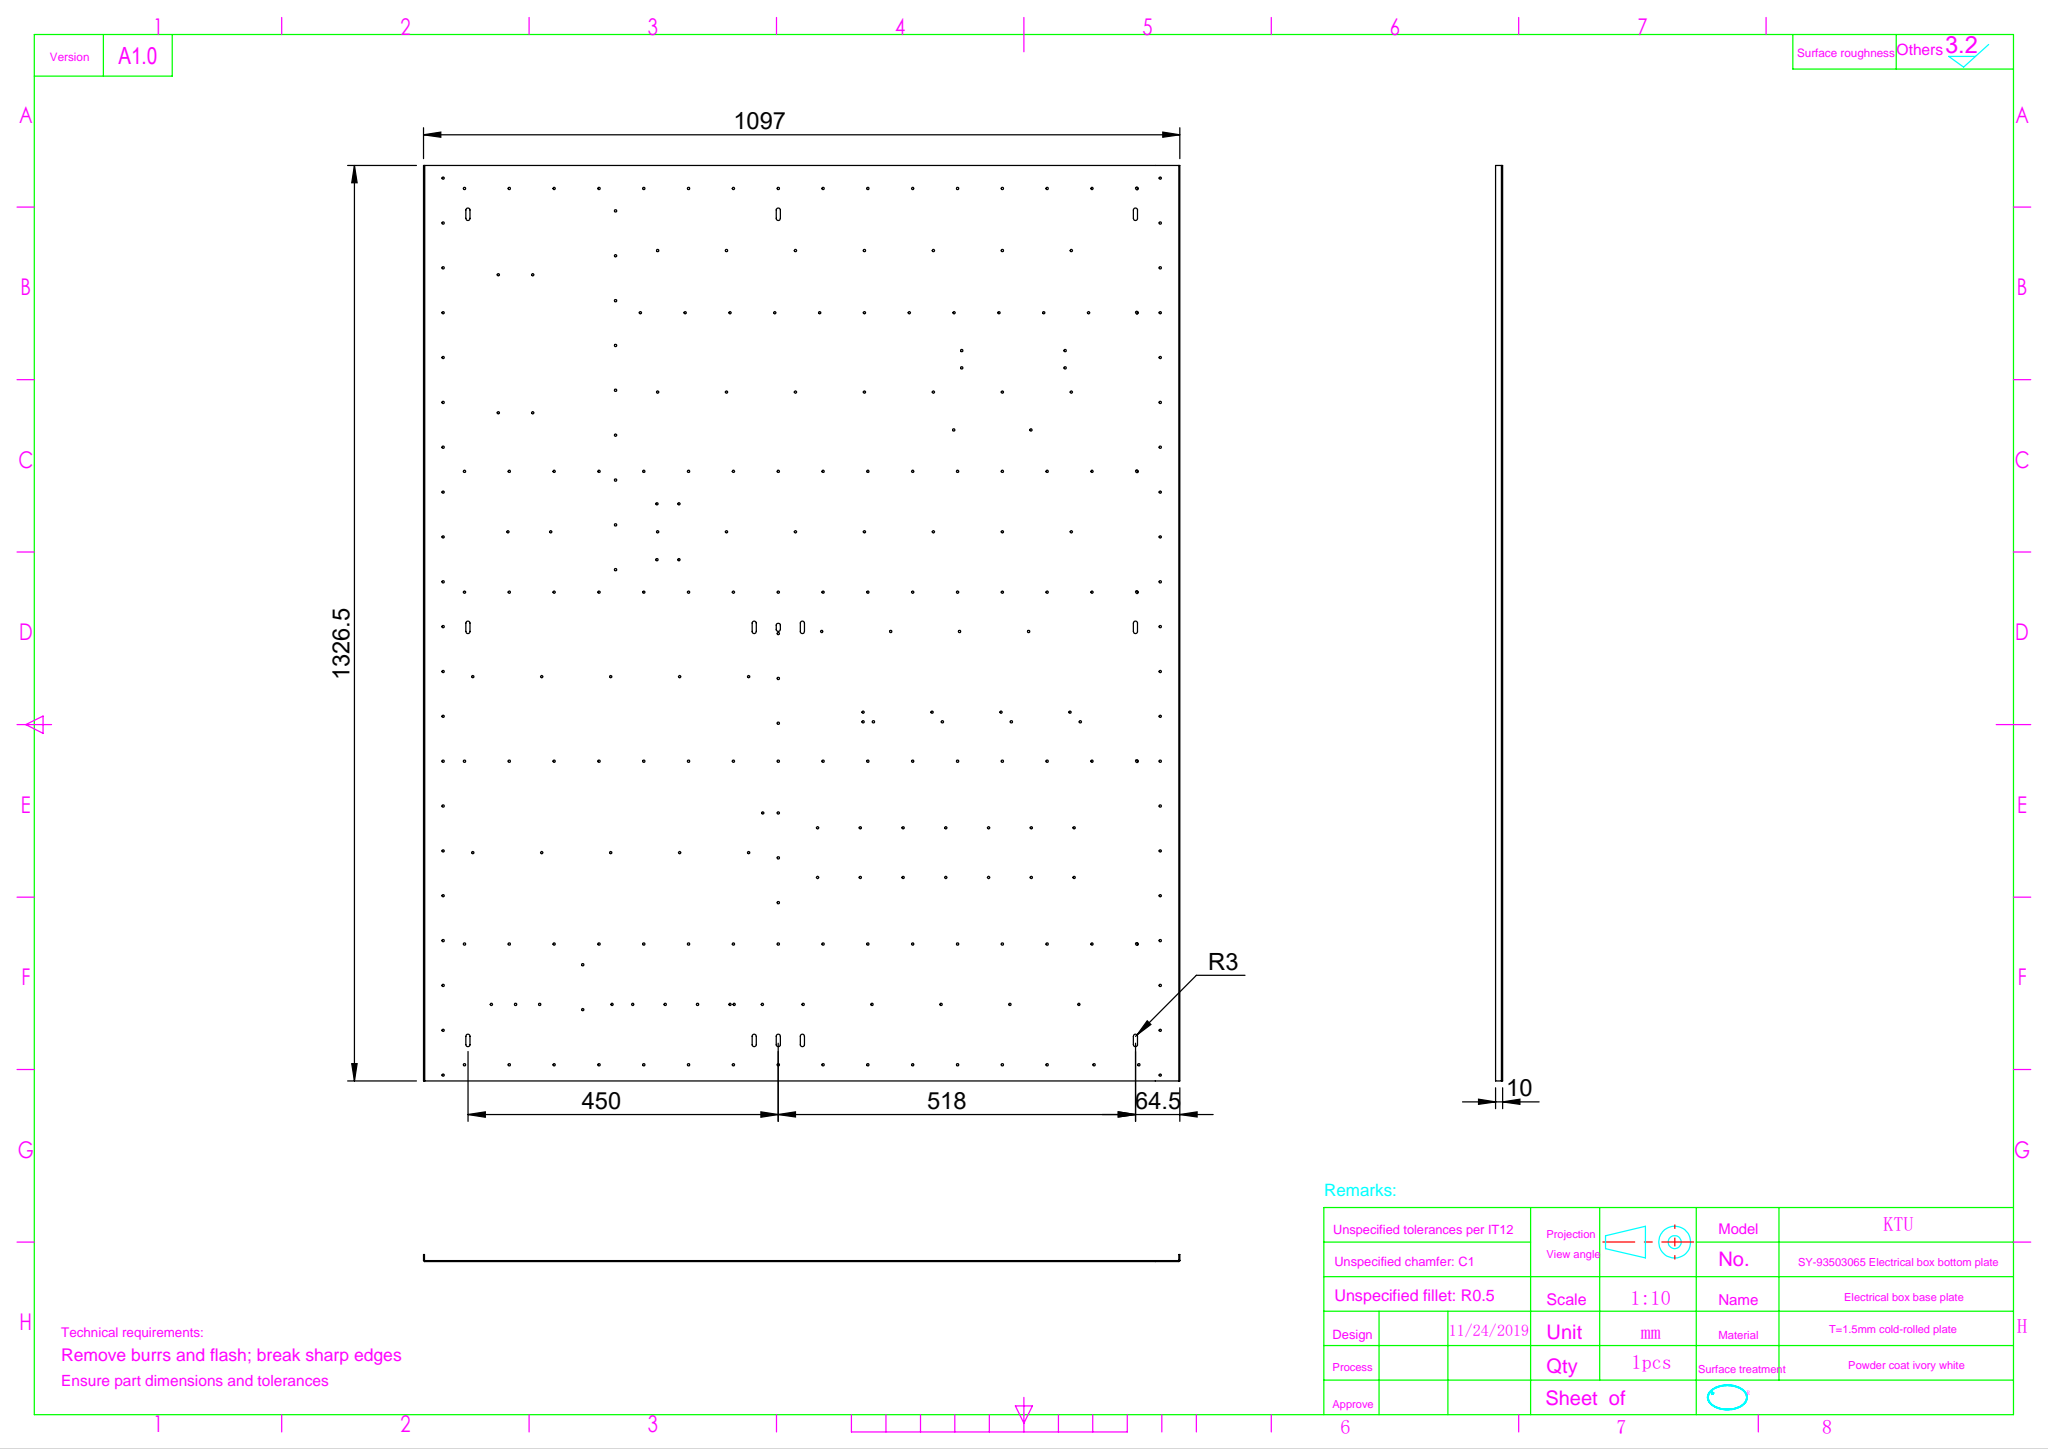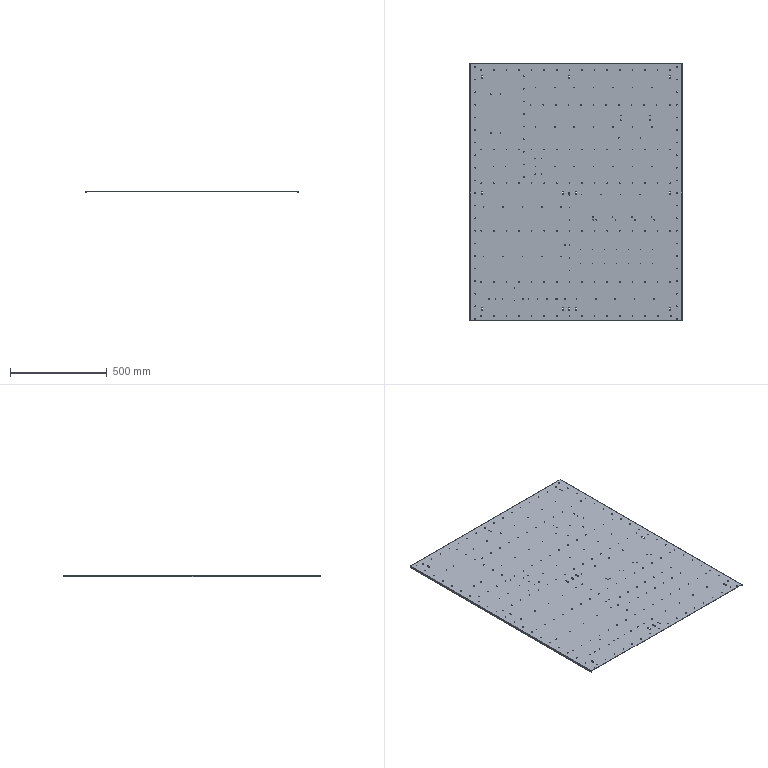Part | SolidWorks | features Cut 5, MoveFace 5, EdgeFlange 2, ICE 2, FlatPattern 1, HoleWzd 1, SMBaseFlange 1, SheetMetal 1 | 1 solid | 588 faces | box 1097 x 1327 x 10 mm | volume 2209760 mm3 | cylinder 544 | plane 44 | commonest cylinder face diameters 3.3 x514 6 x26 0.4 x2 3.4 x2